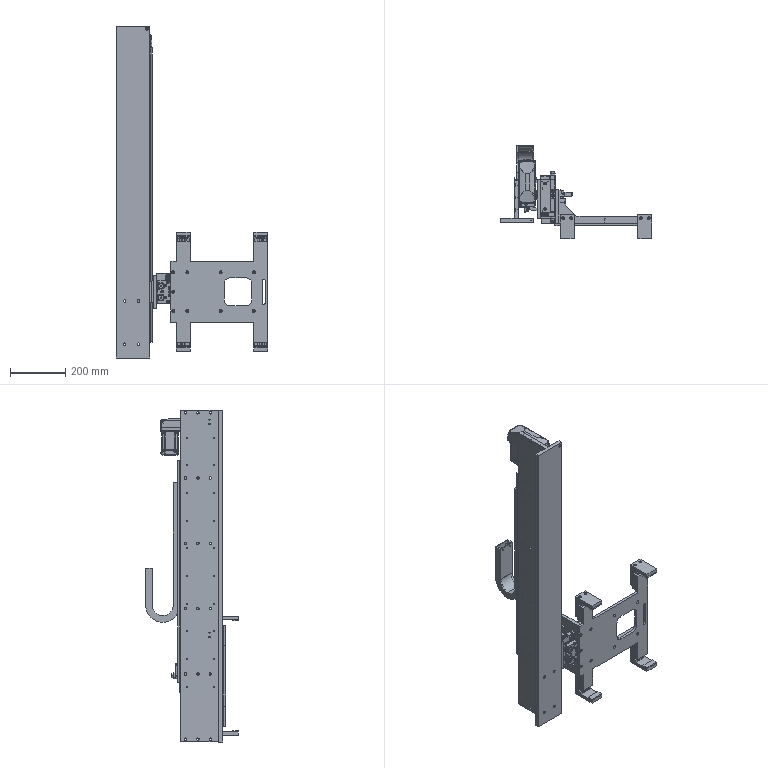Part | SolidWorks | features ReferencePattern 5, LocalLPattern 1 | 45 solids | 4754 faces | volume 11174306 mm3 | cylinder 1953 | plane 1942 | cone 671 | spline 164 | torus 18 | sphere 6 | commonest cylinder face diameters 6 x111 3.242 x96 4 x89 11 x86 4.2 x82 9 x80